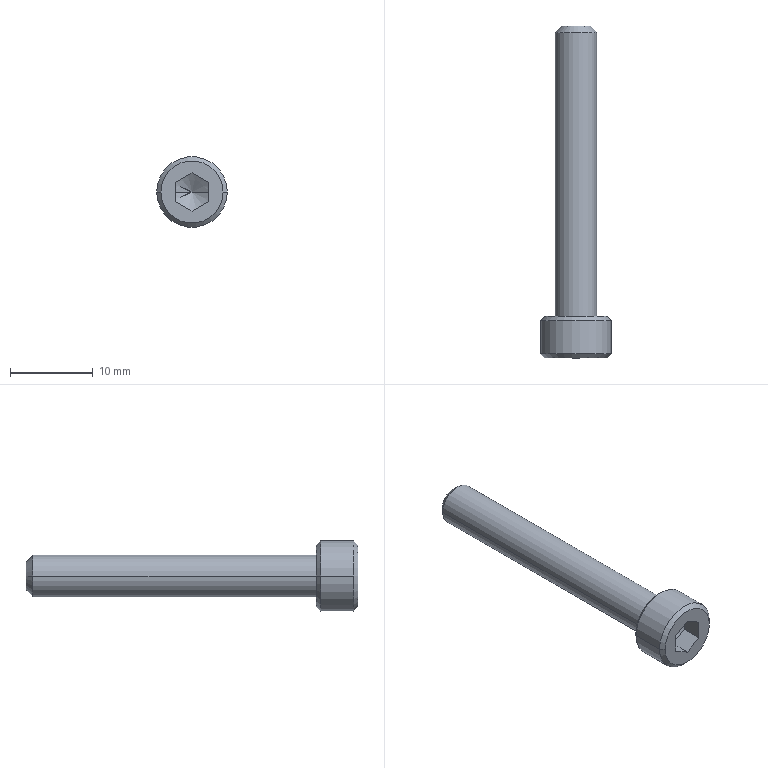Part | STEP file | BB62-M5-35L-3 | 1 solid | 27 faces | box 8.5 x 40 x 8.5 mm | volume 918.722 mm3 | plane 15 | cone 8 | cylinder 4 | commonest cylinder face diameters 5 x2 8.5 x2
STEP:
#1=CARTESIAN_POINT('',(0.,-1.178,0.));
#2=VERTEX_POINT('',#1);
#3=CARTESIAN_POINT('',(2.29,-2.5,0.));
#4=VERTEX_POINT('',#3);
#5=CARTESIAN_POINT('',(0.,-1.178,0.));
#6=DIRECTION('',(0.866,-0.5,0.));
#7=VECTOR('',#6,1000.);
#8=LINE('',#5,#7);
#9=EDGE_CURVE('',#2,#4,#8,.T.);
#10=ORIENTED_EDGE('',*,*,#9,.F.);
#11=CARTESIAN_POINT('',(-2.29,-2.5,0.));
#12=VERTEX_POINT('',#11);
#13=CARTESIAN_POINT('',(0.,-1.178,0.));
#14=DIRECTION('',(-0.866,-0.5,0.));
#15=VECTOR('',#14,1000.);
#16=LINE('',#13,#15);
#17=EDGE_CURVE('',#2,#12,#16,.T.);
#18=ORIENTED_EDGE('',*,*,#17,.T.);
#19=CARTESIAN_POINT('',(-1.983,-2.5,-1.145));
#20=VERTEX_POINT('',#19);
#21=CARTESIAN_POINT('',(0.,-2.5,0.));
#22=DIRECTION('',(0.,-1.,0.));
#23=DIRECTION('',(-1.,0.,0.));
#24=AXIS2_PLACEMENT_3D('',#21,#22,#23);
#25=CIRCLE('',#24,2.29);
#26=EDGE_CURVE('',#12,#20,#25,.T.);
#27=ORIENTED_EDGE('',*,*,#26,.T.);
#28=CARTESIAN_POINT('',(0.,-2.5,-2.29));
#29=VERTEX_POINT('',#28);
#30=CARTESIAN_POINT('',(0.,-2.5,0.));
#31=DIRECTION('',(0.,-1.,0.));
#32=DIRECTION('',(-1.,0.,0.));
#33=AXIS2_PLACEMENT_3D('',#30,#31,#32);
#34=CIRCLE('',#33,2.29);
#35=EDGE_CURVE('',#20,#29,#34,.T.);
#36=ORIENTED_EDGE('',*,*,#35,.T.);
#37=CARTESIAN_POINT('',(1.983,-2.5,-1.145));
#38=VERTEX_POINT('',#37);
#39=CARTESIAN_POINT('',(0.,-2.5,0.));
#40=DIRECTION('',(0.,-1.,0.));
#41=DIRECTION('',(-1.,0.,0.));
#42=AXIS2_PLACEMENT_3D('',#39,#40,#41);
#43=CIRCLE('',#42,2.29);
#44=EDGE_CURVE('',#29,#38,#43,.T.);
#45=ORIENTED_EDGE('',*,*,#44,.T.);
#46=CARTESIAN_POINT('',(0.,-2.5,0.));
#47=DIRECTION('',(0.,-1.,0.));
#48=DIRECTION('',(-1.,0.,0.));
#49=AXIS2_PLACEMENT_3D('',#46,#47,#48);
#50=CIRCLE('',#49,2.29);
#51=EDGE_CURVE('',#38,#4,#50,.T.);
#52=ORIENTED_EDGE('',*,*,#51,.T.);
#53=EDGE_LOOP('',(#10,#18,#27,#36,#45,#52));
#54=FACE_OUTER_BOUND('',#53,.T.);
#55=CARTESIAN_POINT('',(0.,-1001.178,0.));
#56=DIRECTION('',(0.,-1.,0.));
#57=DIRECTION('',(1.,0.,0.));
#58=AXIS2_PLACEMENT_3D('',#55,#56,#57);
#59=CONICAL_SURFACE('',#58,1732.051,1.047);
#60=ADVANCED_FACE('',(#54),#59,.F.);
#61=CARTESIAN_POINT('',(-1.7,35.,0.));
#62=VERTEX_POINT('',#61);
#63=CARTESIAN_POINT('',(1.7,35.,0.));
#64=VERTEX_POINT('',#63);
#65=CARTESIAN_POINT('',(0.,35.,0.));
#66=DIRECTION('',(0.,1.,0.));
#67=DIRECTION('',(1.,0.,0.));
#68=AXIS2_PLACEMENT_3D('',#65,#66,#67);
#69=CIRCLE('',#68,1.7);
#70=EDGE_CURVE('',#62,#64,#69,.T.);
#71=ORIENTED_EDGE('',*,*,#70,.F.);
#72=CARTESIAN_POINT('',(-2.5,34.2,0.));
#73=VERTEX_POINT('',#72);
#74=CARTESIAN_POINT('',(-1.7,35.,0.));
#75=DIRECTION('',(-0.7071,-0.7071,0.));
#76=VECTOR('',#75,1000.);
#77=LINE('',#74,#76);
#78=EDGE_CURVE('',#62,#73,#77,.T.);
#79=ORIENTED_EDGE('',*,*,#78,.T.);
#80=CARTESIAN_POINT('',(2.5,34.2,0.));
#81=VERTEX_POINT('',#80);
#82=CARTESIAN_POINT('',(0.,34.2,0.));
#83=DIRECTION('',(0.,-1.,0.));
#84=DIRECTION('',(-1.,0.,0.));
#85=AXIS2_PLACEMENT_3D('',#82,#83,#84);
#86=CIRCLE('',#85,2.5);
#87=EDGE_CURVE('',#81,#73,#86,.T.);
#88=ORIENTED_EDGE('',*,*,#87,.F.);
#89=CARTESIAN_POINT('',(1.7,35.,0.));
#90=DIRECTION('',(0.7071,-0.7071,0.));
#91=VECTOR('',#90,1000.);
#92=LINE('',#89,#91);
#93=EDGE_CURVE('',#64,#81,#92,.T.);
#94=ORIENTED_EDGE('',*,*,#93,.F.);
#95=EDGE_LOOP('',(#71,#79,#88,#94));
#96=FACE_OUTER_BOUND('',#95,.T.);
#97=CARTESIAN_POINT('',(0.,35.,0.));
#98=DIRECTION('',(0.,-1.,0.));
#99=DIRECTION('',(1.,0.,0.));
#100=AXIS2_PLACEMENT_3D('',#97,#98,#99);
#101=CONICAL_SURFACE('',#100,1.7,0.7854);
#102=ADVANCED_FACE('',(#96),#101,.T.);
#103=ORIENTED_EDGE('',*,*,#87,.T.);
#104=CARTESIAN_POINT('',(-2.5,0.,0.));
#105=VERTEX_POINT('',#104);
#106=CARTESIAN_POINT('',(-2.5,34.2,0.));
#107=DIRECTION('',(0.,-1.,0.));
#108=VECTOR('',#107,1000.);
#109=LINE('',#106,#108);
#110=EDGE_CURVE('',#73,#105,#109,.T.);
#111=ORIENTED_EDGE('',*,*,#110,.T.);
#112=CARTESIAN_POINT('',(2.5,0.,0.));
#113=VERTEX_POINT('',#112);
#114=CARTESIAN_POINT('',(0.,0.,0.));
#115=DIRECTION('',(0.,-1.,0.));
#116=DIRECTION('',(-1.,0.,0.));
#117=AXIS2_PLACEMENT_3D('',#114,#115,#116);
#118=CIRCLE('',#117,2.5);
#119=EDGE_CURVE('',#113,#105,#118,.T.);
#120=ORIENTED_EDGE('',*,*,#119,.F.);
#121=CARTESIAN_POINT('',(2.5,34.2,0.));
#122=DIRECTION('',(0.,-1.,0.));
#123=VECTOR('',#122,1000.);
#124=LINE('',#121,#123);
#125=EDGE_CURVE('',#81,#113,#124,.T.);
#126=ORIENTED_EDGE('',*,*,#125,.F.);
#127=EDGE_LOOP('',(#103,#111,#120,#126));
#128=FACE_OUTER_BOUND('',#127,.T.);
#129=CARTESIAN_POINT('',(0.,34.2,0.));
#130=DIRECTION('',(0.,-1.,0.));
#131=DIRECTION('',(1.,0.,0.));
#132=AXIS2_PLACEMENT_3D('',#129,#130,#131);
#133=CYLINDRICAL_SURFACE('',#132,2.5);
#134=ADVANCED_FACE('',(#128),#133,.T.);
#135=CARTESIAN_POINT('',(3.75,-5.,0.));
#136=VERTEX_POINT('',#135);
#137=CARTESIAN_POINT('',(-3.75,-5.,0.));
#138=VERTEX_POINT('',#137);
#139=CARTESIAN_POINT('',(0.,-5.,0.));
#140=DIRECTION('',(0.,-1.,0.));
#141=DIRECTION('',(-1.,0.,0.));
#142=AXIS2_PLACEMENT_3D('',#139,#140,#141);
#143=CIRCLE('',#142,3.75);
#144=EDGE_CURVE('',#136,#138,#143,.T.);
#145=ORIENTED_EDGE('',*,*,#144,.F.);
#146=CARTESIAN_POINT('',(4.25,-4.5,0.));
#147=VERTEX_POINT('',#146);
#148=CARTESIAN_POINT('',(4.25,-4.5,0.));
#149=DIRECTION('',(0.7071,0.7071,0.));
#150=VECTOR('',#149,1000.);
#151=LINE('',#148,#150);
#152=EDGE_CURVE('',#136,#147,#151,.T.);
#153=ORIENTED_EDGE('',*,*,#152,.T.);
#154=CARTESIAN_POINT('',(-4.25,-4.5,0.));
#155=VERTEX_POINT('',#154);
#156=CARTESIAN_POINT('',(0.,-4.5,0.));
#157=DIRECTION('',(0.,-1.,0.));
#158=DIRECTION('',(-1.,0.,0.));
#159=AXIS2_PLACEMENT_3D('',#156,#157,#158);
#160=CIRCLE('',#159,4.25);
#161=EDGE_CURVE('',#147,#155,#160,.T.);
#162=ORIENTED_EDGE('',*,*,#161,.T.);
#163=CARTESIAN_POINT('',(-4.25,-4.5,0.));
#164=DIRECTION('',(-0.7071,0.7071,0.));
#165=VECTOR('',#164,1000.);
#166=LINE('',#163,#165);
#167=EDGE_CURVE('',#138,#155,#166,.T.);
#168=ORIENTED_EDGE('',*,*,#167,.F.);
#169=EDGE_LOOP('',(#145,#153,#162,#168));
#170=FACE_OUTER_BOUND('',#169,.T.);
#171=CARTESIAN_POINT('',(0.,-4.5,0.));
#172=DIRECTION('',(0.,1.,0.));
#173=DIRECTION('',(-1.,0.,0.));
#174=AXIS2_PLACEMENT_3D('',#171,#172,#173);
#175=CONICAL_SURFACE('',#174,4.25,0.7854);
#176=ADVANCED_FACE('',(#170),#175,.T.);
#177=ORIENTED_EDGE('',*,*,#161,.F.);
#178=CARTESIAN_POINT('',(4.25,-0.5,0.));
#179=VERTEX_POINT('',#178);
#180=CARTESIAN_POINT('',(4.25,-1.62,0.));
#181=DIRECTION('',(0.,1.,0.));
#182=VECTOR('',#181,1000.);
#183=LINE('',#180,#182);
#184=EDGE_CURVE('',#147,#179,#183,.T.);
#185=ORIENTED_EDGE('',*,*,#184,.T.);
#186=CARTESIAN_POINT('',(-4.25,-0.5,0.));
#187=VERTEX_POINT('',#186);
#188=CARTESIAN_POINT('',(0.,-0.5,0.));
#189=DIRECTION('',(0.,-1.,0.));
#190=DIRECTION('',(-1.,0.,0.));
#191=AXIS2_PLACEMENT_3D('',#188,#189,#190);
#192=CIRCLE('',#191,4.25);
#193=EDGE_CURVE('',#179,#187,#192,.T.);
#194=ORIENTED_EDGE('',*,*,#193,.T.);
#195=CARTESIAN_POINT('',(-4.25,-1.62,0.));
#196=DIRECTION('',(0.,1.,0.));
#197=VECTOR('',#196,1000.);
#198=LINE('',#195,#197);
#199=EDGE_CURVE('',#155,#187,#198,.T.);
#200=ORIENTED_EDGE('',*,*,#199,.F.);
#201=EDGE_LOOP('',(#177,#185,#194,#200));
#202=FACE_OUTER_BOUND('',#201,.T.);
#203=CARTESIAN_POINT('',(0.,-1.62,0.));
#204=DIRECTION('',(0.,1.,0.));
#205=DIRECTION('',(-1.,0.,0.));
#206=AXIS2_PLACEMENT_3D('',#203,#204,#205);
#207=CYLINDRICAL_SURFACE('',#206,4.25);
#208=ADVANCED_FACE('',(#202),#207,.T.);
#209=CARTESIAN_POINT('',(3.75,0.,0.));
#210=VERTEX_POINT('',#209);
#211=CARTESIAN_POINT('',(-3.75,0.,0.));
#212=VERTEX_POINT('',#211);
#213=CARTESIAN_POINT('',(0.,0.,0.));
#214=DIRECTION('',(0.,-1.,0.));
#215=DIRECTION('',(-1.,0.,0.));
#216=AXIS2_PLACEMENT_3D('',#213,#214,#215);
#217=CIRCLE('',#216,3.75);
#218=EDGE_CURVE('',#210,#212,#217,.T.);
#219=ORIENTED_EDGE('',*,*,#218,.T.);
#220=CARTESIAN_POINT('',(-3.75,0.,0.));
#221=DIRECTION('',(-0.7071,-0.7071,0.));
#222=VECTOR('',#221,1000.);
#223=LINE('',#220,#222);
#224=EDGE_CURVE('',#212,#187,#223,.T.);
#225=ORIENTED_EDGE('',*,*,#224,.T.);
#226=ORIENTED_EDGE('',*,*,#193,.F.);
#227=CARTESIAN_POINT('',(3.75,0.,0.));
#228=DIRECTION('',(0.7071,-0.7071,0.));
#229=VECTOR('',#228,1000.);
#230=LINE('',#227,#229);
#231=EDGE_CURVE('',#210,#179,#230,.T.);
#232=ORIENTED_EDGE('',*,*,#231,.F.);
#233=EDGE_LOOP('',(#219,#225,#226,#232));
#234=FACE_OUTER_BOUND('',#233,.T.);
#235=CARTESIAN_POINT('',(0.,0.,0.));
#236=DIRECTION('',(0.,-1.,0.));
#237=DIRECTION('',(1.,0.,0.));
#238=AXIS2_PLACEMENT_3D('',#235,#236,#237);
#239=CONICAL_SURFACE('',#238,3.75,0.7854);
#240=ADVANCED_FACE('',(#234),#239,.T.);
#241=CARTESIAN_POINT('',(0.,-5.,0.));
#242=DIRECTION('',(0.,-1.,0.));
#243=DIRECTION('',(-1.,0.,0.));
#244=AXIS2_PLACEMENT_3D('',#241,#242,#243);
#245=CIRCLE('',#244,3.75);
#246=EDGE_CURVE('',#138,#136,#245,.T.);
#247=ORIENTED_EDGE('',*,*,#246,.T.);
#248=ORIENTED_EDGE('',*,*,#144,.T.);
#249=EDGE_LOOP('',(#247,#248));
#250=FACE_OUTER_BOUND('',#249,.T.);
#251=CARTESIAN_POINT('',(0.,-5.,-2.29));
#252=VERTEX_POINT('',#251);
#253=CARTESIAN_POINT('',(-1.983,-5.,-1.145));
#254=VERTEX_POINT('',#253);
#255=CARTESIAN_POINT('',(0.,-5.,-2.29));
#256=DIRECTION('',(-0.866,0.,0.5));
#257=VECTOR('',#256,1000.);
#258=LINE('',#255,#257);
#259=EDGE_CURVE('',#252,#254,#258,.T.);
#260=ORIENTED_EDGE('',*,*,#259,.T.);
#261=CARTESIAN_POINT('',(-1.983,-5.,1.145));
#262=VERTEX_POINT('',#261);
#263=CARTESIAN_POINT('',(-1.983,-5.,-1.145));
#264=DIRECTION('',(0.,0.,1.));
#265=VECTOR('',#264,1000.);
#266=LINE('',#263,#265);
#267=EDGE_CURVE('',#254,#262,#266,.T.);
#268=ORIENTED_EDGE('',*,*,#267,.T.);
#269=CARTESIAN_POINT('',(0.,-5.,2.29));
#270=VERTEX_POINT('',#269);
#271=CARTESIAN_POINT('',(-1.983,-5.,1.145));
#272=DIRECTION('',(0.866,0.,0.5));
#273=VECTOR('',#272,1000.);
#274=LINE('',#271,#273);
#275=EDGE_CURVE('',#262,#270,#274,.T.);
#276=ORIENTED_EDGE('',*,*,#275,.T.);
#277=CARTESIAN_POINT('',(1.983,-5.,1.145));
#278=VERTEX_POINT('',#277);
#279=CARTESIAN_POINT('',(0.,-5.,2.29));
#280=DIRECTION('',(0.866,0.,-0.5));
#281=VECTOR('',#280,1000.);
#282=LINE('',#279,#281);
#283=EDGE_CURVE('',#270,#278,#282,.T.);
#284=ORIENTED_EDGE('',*,*,#283,.T.);
#285=CARTESIAN_POINT('',(1.983,-5.,-1.145));
#286=VERTEX_POINT('',#285);
#287=CARTESIAN_POINT('',(1.983,-5.,1.145));
#288=DIRECTION('',(0.,0.,-1.));
#289=VECTOR('',#288,1000.);
#290=LINE('',#287,#289);
#291=EDGE_CURVE('',#278,#286,#290,.T.);
#292=ORIENTED_EDGE('',*,*,#291,.T.);
#293=CARTESIAN_POINT('',(1.983,-5.,-1.145));
#294=DIRECTION('',(-0.866,0.,-0.5));
#295=VECTOR('',#294,1000.);
#296=LINE('',#293,#295);
#297=EDGE_CURVE('',#286,#252,#296,.T.);
#298=ORIENTED_EDGE('',*,*,#297,.T.);
#299=EDGE_LOOP('',(#260,#268,#276,#284,#292,#298));
#300=FACE_BOUND('',#299,.T.);
#301=CARTESIAN_POINT('',(3.75,-5.,0.));
#302=DIRECTION('',(0.,-1.,0.));
#303=DIRECTION('',(1.,0.,0.));
#304=AXIS2_PLACEMENT_3D('',#301,#302,#303);
#305=PLANE('',#304);
#306=ADVANCED_FACE('',(#250,#300),#305,.T.);
#307=ORIENTED_EDGE('',*,*,#119,.T.);
#308=CARTESIAN_POINT('',(0.,0.,0.));
#309=DIRECTION('',(0.,-1.,0.));
#310=DIRECTION('',(-1.,0.,0.));
#311=AXIS2_PLACEMENT_3D('',#308,#309,#310);
#312=CIRCLE('',#311,2.5);
#313=EDGE_CURVE('',#105,#113,#312,.T.);
#314=ORIENTED_EDGE('',*,*,#313,.T.);
#315=EDGE_LOOP('',(#307,#314));
#316=FACE_BOUND('',#315,.T.);
#317=ORIENTED_EDGE('',*,*,#218,.F.);
#318=CARTESIAN_POINT('',(0.,0.,0.));
#319=DIRECTION('',(0.,-1.,0.));
#320=DIRECTION('',(-1.,0.,0.));
#321=AXIS2_PLACEMENT_3D('',#318,#319,#320);
#322=CIRCLE('',#321,3.75);
#323=EDGE_CURVE('',#212,#210,#322,.T.);
#324=ORIENTED_EDGE('',*,*,#323,.F.);
#325=EDGE_LOOP('',(#317,#324));
#326=FACE_OUTER_BOUND('',#325,.T.);
#327=CARTESIAN_POINT('',(0.,0.,0.));
#328=DIRECTION('',(0.,1.,0.));
#329=DIRECTION('',(-1.,0.,0.));
#330=AXIS2_PLACEMENT_3D('',#327,#328,#329);
#331=PLANE('',#330);
#332=ADVANCED_FACE('',(#316,#326),#331,.T.);
#333=ORIENTED_EDGE('',*,*,#224,.F.);
#334=ORIENTED_EDGE('',*,*,#323,.T.);
#335=ORIENTED_EDGE('',*,*,#231,.T.);
#336=CARTESIAN_POINT('',(0.,-0.5,0.));
#337=DIRECTION('',(0.,-1.,0.));
#338=DIRECTION('',(-1.,0.,0.));
#339=AXIS2_PLACEMENT_3D('',#336,#337,#338);
#340=CIRCLE('',#339,4.25);
#341=EDGE_CURVE('',#187,#179,#340,.T.);
#342=ORIENTED_EDGE('',*,*,#341,.F.);
#343=EDGE_LOOP('',(#333,#334,#335,#342));
#344=FACE_OUTER_BOUND('',#343,.T.);
#345=CARTESIAN_POINT('',(0.,0.,0.));
#346=DIRECTION('',(0.,-1.,0.));
#347=DIRECTION('',(1.,0.,0.));
#348=AXIS2_PLACEMENT_3D('',#345,#346,#347);
#349=CONICAL_SURFACE('',#348,3.75,0.7854);
#350=ADVANCED_FACE('',(#344),#349,.T.);
#351=ORIENTED_EDGE('',*,*,#184,.F.);
#352=CARTESIAN_POINT('',(0.,-4.5,0.));
#353=DIRECTION('',(0.,-1.,0.));
#354=DIRECTION('',(-1.,0.,0.));
#355=AXIS2_PLACEMENT_3D('',#352,#353,#354);
#356=CIRCLE('',#355,4.25);
#357=EDGE_CURVE('',#155,#147,#356,.T.);
#358=ORIENTED_EDGE('',*,*,#357,.F.);
#359=ORIENTED_EDGE('',*,*,#199,.T.);
#360=ORIENTED_EDGE('',*,*,#341,.T.);
#361=EDGE_LOOP('',(#351,#358,#359,#360));
#362=FACE_OUTER_BOUND('',#361,.T.);
#363=CARTESIAN_POINT('',(0.,-1.62,0.));
#364=DIRECTION('',(0.,1.,0.));
#365=DIRECTION('',(-1.,0.,0.));
#366=AXIS2_PLACEMENT_3D('',#363,#364,#365);
#367=CYLINDRICAL_SURFACE('',#366,4.25);
#368=ADVANCED_FACE('',(#362),#367,.T.);
#369=ORIENTED_EDGE('',*,*,#152,.F.);
#370=ORIENTED_EDGE('',*,*,#246,.F.);
#371=ORIENTED_EDGE('',*,*,#167,.T.);
#372=ORIENTED_EDGE('',*,*,#357,.T.);
#373=EDGE_LOOP('',(#369,#370,#371,#372));
#374=FACE_OUTER_BOUND('',#373,.T.);
#375=CARTESIAN_POINT('',(0.,-4.5,0.));
#376=DIRECTION('',(0.,1.,0.));
#377=DIRECTION('',(-1.,0.,0.));
#378=AXIS2_PLACEMENT_3D('',#375,#376,#377);
#379=CONICAL_SURFACE('',#378,4.25,0.7854);
#380=ADVANCED_FACE('',(#374),#379,.T.);
#381=ORIENTED_EDGE('',*,*,#110,.F.);
#382=CARTESIAN_POINT('',(0.,34.2,0.));
#383=DIRECTION('',(0.,-1.,0.));
#384=DIRECTION('',(-1.,0.,0.));
#385=AXIS2_PLACEMENT_3D('',#382,#383,#384);
#386=CIRCLE('',#385,2.5);
#387=EDGE_CURVE('',#73,#81,#386,.T.);
#388=ORIENTED_EDGE('',*,*,#387,.T.);
#389=ORIENTED_EDGE('',*,*,#125,.T.);
#390=ORIENTED_EDGE('',*,*,#313,.F.);
#391=EDGE_LOOP('',(#381,#388,#389,#390));
#392=FACE_OUTER_BOUND('',#391,.T.);
#393=CARTESIAN_POINT('',(0.,34.2,0.));
#394=DIRECTION('',(0.,-1.,0.));
#395=DIRECTION('',(1.,0.,0.));
#396=AXIS2_PLACEMENT_3D('',#393,#394,#395);
#397=CYLINDRICAL_SURFACE('',#396,2.5);
#398=ADVANCED_FACE('',(#392),#397,.T.);
#399=CARTESIAN_POINT('',(0.,35.,0.));
#400=DIRECTION('',(0.,1.,0.));
#401=DIRECTION('',(1.,0.,0.));
#402=AXIS2_PLACEMENT_3D('',#399,#400,#401);
#403=CIRCLE('',#402,1.7);
#404=EDGE_CURVE('',#64,#62,#403,.T.);
#405=ORIENTED_EDGE('',*,*,#404,.T.);
#406=ORIENTED_EDGE('',*,*,#70,.T.);
#407=EDGE_LOOP('',(#405,#406));
#408=FACE_OUTER_BOUND('',#407,.T.);
#409=CARTESIAN_POINT('',(0.,35.,0.));
#410=DIRECTION('',(0.,1.,0.));
#411=DIRECTION('',(-1.,0.,0.));
#412=AXIS2_PLACEMENT_3D('',#409,#410,#411);
#413=PLANE('',#412);
#414=ADVANCED_FACE('',(#408),#413,.T.);
#415=ORIENTED_EDGE('',*,*,#78,.F.);
#416=ORIENTED_EDGE('',*,*,#404,.F.);
#417=ORIENTED_EDGE('',*,*,#93,.T.);
#418=ORIENTED_EDGE('',*,*,#387,.F.);
#419=EDGE_LOOP('',(#415,#416,#417,#418));
#420=FACE_OUTER_BOUND('',#419,.T.);
#421=CARTESIAN_POINT('',(0.,35.,0.));
#422=DIRECTION('',(0.,-1.,0.));
#423=DIRECTION('',(1.,0.,0.));
#424=AXIS2_PLACEMENT_3D('',#421,#422,#423);
#425=CONICAL_SURFACE('',#424,1.7,0.7854);
#426=ADVANCED_FACE('',(#420),#425,.T.);
#427=CARTESIAN_POINT('',(1.983,-2.5,-1.145));
#428=DIRECTION('',(-0.866,0.,-0.5));
#429=VECTOR('',#428,1000.);
#430=LINE('',#427,#429);
#431=EDGE_CURVE('',#38,#29,#430,.T.);
#432=ORIENTED_EDGE('',*,*,#431,.T.);
#433=CARTESIAN_POINT('',(0.,-5.,-2.29));
#434=DIRECTION('',(0.,1.,0.));
#435=VECTOR('',#434,1000.);
#436=LINE('',#433,#435);
#437=EDGE_CURVE('',#252,#29,#436,.T.);
#438=ORIENTED_EDGE('',*,*,#437,.F.);
#439=ORIENTED_EDGE('',*,*,#297,.F.);
#440=CARTESIAN_POINT('',(1.983,-5.,-1.145));
#441=DIRECTION('',(0.,1.,0.));
#442=VECTOR('',#441,1000.);
#443=LINE('',#440,#442);
#444=EDGE_CURVE('',#286,#38,#443,.T.);
#445=ORIENTED_EDGE('',*,*,#444,.T.);
#446=EDGE_LOOP('',(#432,#438,#439,#445));
#447=FACE_OUTER_BOUND('',#446,.T.);
#448=CARTESIAN_POINT('',(1.983,-5.,-1.145));
#449=DIRECTION('',(-0.5,0.,0.866));
#450=DIRECTION('',(0.866,0.,0.5));
#451=AXIS2_PLACEMENT_3D('',#448,#449,#450);
#452=PLANE('',#451);
#453=ADVANCED_FACE('',(#447),#452,.T.);
#454=CARTESIAN_POINT('',(0.,-2.5,-2.29));
#455=DIRECTION('',(-0.866,0.,0.5));
#456=VECTOR('',#455,1000.);
#457=LINE('',#454,#456);
#458=EDGE_CURVE('',#29,#20,#457,.T.);
#459=ORIENTED_EDGE('',*,*,#458,.T.);
#460=CARTESIAN_POINT('',(-1.983,-5.,-1.145));
#461=DIRECTION('',(0.,1.,0.));
#462=VECTOR('',#461,1000.);
#463=LINE('',#460,#462);
#464=EDGE_CURVE('',#254,#20,#463,.T.);
#465=ORIENTED_EDGE('',*,*,#464,.F.);
#466=ORIENTED_EDGE('',*,*,#259,.F.);
#467=ORIENTED_EDGE('',*,*,#437,.T.);
#468=EDGE_LOOP('',(#459,#465,#466,#467));
#469=FACE_OUTER_BOUND('',#468,.T.);
#470=CARTESIAN_POINT('',(0.,-5.,-2.29));
#471=DIRECTION('',(0.5,0.,0.866));
#472=DIRECTION('',(0.866,0.,-0.5));
#473=AXIS2_PLACEMENT_3D('',#470,#471,#472);
#474=PLANE('',#473);
#475=ADVANCED_FACE('',(#469),#474,.T.);
#476=CARTESIAN_POINT('',(-1.983,-2.5,1.145));
#477=VERTEX_POINT('',#476);
#478=CARTESIAN_POINT('',(-1.983,-2.5,-1.145));
#479=DIRECTION('',(0.,0.,1.));
#480=VECTOR('',#479,1000.);
#481=LINE('',#478,#480);
#482=EDGE_CURVE('',#20,#477,#481,.T.);
#483=ORIENTED_EDGE('',*,*,#482,.T.);
#484=CARTESIAN_POINT('',(-1.983,-5.,1.145));
#485=DIRECTION('',(0.,1.,0.));
#486=VECTOR('',#485,1000.);
#487=LINE('',#484,#486);
#488=EDGE_CURVE('',#262,#477,#487,.T.);
#489=ORIENTED_EDGE('',*,*,#488,.F.);
#490=ORIENTED_EDGE('',*,*,#267,.F.);
#491=ORIENTED_EDGE('',*,*,#464,.T.);
#492=EDGE_LOOP('',(#483,#489,#490,#491));
#493=FACE_OUTER_BOUND('',#492,.T.);
#494=CARTESIAN_POINT('',(-1.983,-5.,-1.145));
#495=DIRECTION('',(1.,0.,0.));
#496=DIRECTION('',(0.,0.,-1.));
#497=AXIS2_PLACEMENT_3D('',#494,#495,#496);
#498=PLANE('',#497);
#499=ADVANCED_FACE('',(#493),#498,.T.);
#500=CARTESIAN_POINT('',(0.,-2.5,2.29));
#501=VERTEX_POINT('',#500);
#502=CARTESIAN_POINT('',(-1.983,-2.5,1.145));
#503=DIRECTION('',(0.866,0.,0.5));
#504=VECTOR('',#503,1000.);
#505=LINE('',#502,#504);
#506=EDGE_CURVE('',#477,#501,#505,.T.);
#507=ORIENTED_EDGE('',*,*,#506,.T.);
#508=CARTESIAN_POINT('',(0.,-5.,2.29));
#509=DIRECTION('',(0.,1.,0.));
#510=VECTOR('',#509,1000.);
#511=LINE('',#508,#510);
#512=EDGE_CURVE('',#270,#501,#511,.T.);
#513=ORIENTED_EDGE('',*,*,#512,.F.);
#514=ORIENTED_EDGE('',*,*,#275,.F.);
#515=ORIENTED_EDGE('',*,*,#488,.T.);
#516=EDGE_LOOP('',(#507,#513,#514,#515));
#517=FACE_OUTER_BOUND('',#516,.T.);
#518=CARTESIAN_POINT('',(-1.983,-5.,1.145));
#519=DIRECTION('',(0.5,0.,-0.866));
#520=DIRECTION('',(-0.866,0.,-0.5));
#521=AXIS2_PLACEMENT_3D('',#518,#519,#520);
#522=PLANE('',#521);
#523=ADVANCED_FACE('',(#517),#522,.T.);
#524=CARTESIAN_POINT('',(1.983,-2.5,1.145));
#525=VERTEX_POINT('',#524);
#526=CARTESIAN_POINT('',(0.,-2.5,2.29));
#527=DIRECTION('',(0.866,0.,-0.5));
#528=VECTOR('',#527,1000.);
#529=LINE('',#526,#528);
#530=EDGE_CURVE('',#501,#525,#529,.T.);
#531=ORIENTED_EDGE('',*,*,#530,.T.);
#532=CARTESIAN_POINT('',(1.983,-5.,1.145));
#533=DIRECTION('',(0.,1.,0.));
#534=VECTOR('',#533,1000.);
#535=LINE('',#532,#534);
#536=EDGE_CURVE('',#278,#525,#535,.T.);
#537=ORIENTED_EDGE('',*,*,#536,.F.);
#538=ORIENTED_EDGE('',*,*,#283,.F.);
#539=ORIENTED_EDGE('',*,*,#512,.T.);
#540=EDGE_LOOP('',(#531,#537,#538,#539));
#541=FACE_OUTER_BOUND('',#540,.T.);
#542=CARTESIAN_POINT('',(0.,-5.,2.29));
#543=DIRECTION('',(-0.5,0.,-0.866));
#544=DIRECTION('',(-0.866,0.,0.5));
#545=AXIS2_PLACEMENT_3D('',#542,#543,#544);
#546=PLANE('',#545);
#547=ADVANCED_FACE('',(#541),#546,.T.);
#548=CARTESIAN_POINT('',(1.983,-2.5,1.145));
#549=DIRECTION('',(0.,0.,-1.));
#550=VECTOR('',#549,1000.);
#551=LINE('',#548,#550);
#552=EDGE_CURVE('',#525,#38,#551,.T.);
#553=ORIENTED_EDGE('',*,*,#552,.T.);
#554=ORIENTED_EDGE('',*,*,#444,.F.);
#555=ORIENTED_EDGE('',*,*,#291,.F.);
#556=ORIENTED_EDGE('',*,*,#536,.T.);
#557=EDGE_LOOP('',(#553,#554,#555,#556));
#558=FACE_OUTER_BOUND('',#557,.T.);
#559=CARTESIAN_POINT('',(1.983,-5.,1.145));
#560=DIRECTION('',(-1.,0.,0.));
#561=DIRECTION('',(0.,0.,1.));
#562=AXIS2_PLACEMENT_3D('',#559,#560,#561);
#563=PLANE('',#562);
#564=ADVANCED_FACE('',(#558),#563,.T.);
#565=ORIENTED_EDGE('',*,*,#431,.F.);
#566=ORIENTED_EDGE('',*,*,#44,.F.);
#567=EDGE_LOOP('',(#565,#566));
#568=FACE_OUTER_BOUND('',#567,.T.);
#569=CARTESIAN_POINT('',(0.,-2.5,0.));
#570=DIRECTION('',(0.,-1.,0.));
#571=DIRECTION('',(1.,0.,0.));
#572=AXIS2_PLACEMENT_3D('',#569,#570,#571);
#573=PLANE('',#572);
#574=ADVANCED_FACE('',(#568),#573,.F.);
#575=ORIENTED_EDGE('',*,*,#552,.F.);
#576=CARTESIAN_POINT('',(0.,-2.5,0.));
#577=DIRECTION('',(0.,-1.,0.));
#578=DIRECTION('',(-1.,0.,0.));
#579=AXIS2_PLACEMENT_3D('',#576,#577,#578);
#580=CIRCLE('',#579,2.29);
#581=EDGE_CURVE('',#4,#525,#580,.T.);
#582=ORIENTED_EDGE('',*,*,#581,.F.);
#583=ORIENTED_EDGE('',*,*,#51,.F.);
#584=EDGE_LOOP('',(#575,#582,#583));
#585=FACE_OUTER_BOUND('',#584,.T.);
#586=CARTESIAN_POINT('',(0.,-2.5,0.));
#587=DIRECTION('',(0.,-1.,0.));
#588=DIRECTION('',(1.,0.,0.));
#589=AXIS2_PLACEMENT_3D('',#586,#587,#588);
#590=PLANE('',#589);
#591=ADVANCED_FACE('',(#585),#590,.F.);
#592=ORIENTED_EDGE('',*,*,#530,.F.);
#593=CARTESIAN_POINT('',(0.,-2.5,0.));
#594=DIRECTION('',(0.,-1.,0.));
#595=DIRECTION('',(-1.,0.,0.));
#596=AXIS2_PLACEMENT_3D('',#593,#594,#595);
#597=CIRCLE('',#596,2.29);
#598=EDGE_CURVE('',#525,#501,#597,.T.);
#599=ORIENTED_EDGE('',*,*,#598,.F.);
#600=EDGE_LOOP('',(#592,#599));
#601=FACE_OUTER_BOUND('',#600,.T.);
#602=CARTESIAN_POINT('',(0.,-2.5,0.));
#603=DIRECTION('',(0.,-1.,0.));
#604=DIRECTION('',(1.,0.,0.));
#605=AXIS2_PLACEMENT_3D('',#602,#603,#604);
#606=PLANE('',#605);
#607=ADVANCED_FACE('',(#601),#606,.F.);
#608=ORIENTED_EDGE('',*,*,#506,.F.);
#609=CARTESIAN_POINT('',(0.,-2.5,0.));
#610=DIRECTION('',(0.,-1.,0.));
#611=DIRECTION('',(-1.,0.,0.));
#612=AXIS2_PLACEMENT_3D('',#609,#610,#611);
#613=CIRCLE('',#612,2.29);
#614=EDGE_CURVE('',#501,#477,#613,.T.);
#615=ORIENTED_EDGE('',*,*,#614,.F.);
#616=EDGE_LOOP('',(#608,#615));
#617=FACE_OUTER_BOUND('',#616,.T.);
#618=CARTESIAN_POINT('',(0.,-2.5,0.));
#619=DIRECTION('',(0.,-1.,0.));
#620=DIRECTION('',(1.,0.,0.));
#621=AXIS2_PLACEMENT_3D('',#618,#619,#620);
#622=PLANE('',#621);
#623=ADVANCED_FACE('',(#617),#622,.F.);
#624=ORIENTED_EDGE('',*,*,#482,.F.);
#625=ORIENTED_EDGE('',*,*,#26,.F.);
#626=CARTESIAN_POINT('',(0.,-2.5,0.));
#627=DIRECTION('',(0.,-1.,0.));
#628=DIRECTION('',(-1.,0.,0.));
#629=AXIS2_PLACEMENT_3D('',#626,#627,#628);
#630=CIRCLE('',#629,2.29);
#631=EDGE_CURVE('',#477,#12,#630,.T.);
#632=ORIENTED_EDGE('',*,*,#631,.F.);
#633=EDGE_LOOP('',(#624,#625,#632));
#634=FACE_OUTER_BOUND('',#633,.T.);
#635=CARTESIAN_POINT('',(0.,-2.5,0.));
#636=DIRECTION('',(0.,-1.,0.));
#637=DIRECTION('',(1.,0.,0.));
#638=AXIS2_PLACEMENT_3D('',#635,#636,#637);
#639=PLANE('',#638);
#640=ADVANCED_FACE('',(#634),#639,.F.);
#641=ORIENTED_EDGE('',*,*,#458,.F.);
#642=ORIENTED_EDGE('',*,*,#35,.F.);
#643=EDGE_LOOP('',(#641,#642));
#644=FACE_OUTER_BOUND('',#643,.T.);
#645=CARTESIAN_POINT('',(0.,-2.5,0.));
#646=DIRECTION('',(0.,-1.,0.));
#647=DIRECTION('',(1.,0.,0.));
#648=AXIS2_PLACEMENT_3D('',#645,#646,#647);
#649=PLANE('',#648);
#650=ADVANCED_FACE('',(#644),#649,.F.);
#651=ORIENTED_EDGE('',*,*,#17,.F.);
#652=ORIENTED_EDGE('',*,*,#9,.T.);
#653=ORIENTED_EDGE('',*,*,#581,.T.);
#654=ORIENTED_EDGE('',*,*,#598,.T.);
#655=ORIENTED_EDGE('',*,*,#614,.T.);
#656=ORIENTED_EDGE('',*,*,#631,.T.);
#657=EDGE_LOOP('',(#651,#652,#653,#654,#655,#656));
#658=FACE_OUTER_BOUND('',#657,.T.);
#659=CARTESIAN_POINT('',(0.,-1001.178,0.));
#660=DIRECTION('',(0.,-1.,0.));
#661=DIRECTION('',(1.,0.,0.));
#662=AXIS2_PLACEMENT_3D('',#659,#660,#661);
#663=CONICAL_SURFACE('',#662,1732.051,1.047);
#664=ADVANCED_FACE('',(#658),#663,.F.);
#665=CLOSED_SHELL('',(#60,#102,#134,#176,#208,#240,#306,#332,#350,#368,#380,#398,#414,#426,#453,#475,#499,#523,#547,#564,#574,#591,#607,#623,#640,#650,#664));
#666=MANIFOLD_SOLID_BREP('',#665);
#667=CARTESIAN_POINT('',(0.,0.,0.));
#668=DIRECTION('',(0.,0.,1.));
#669=DIRECTION('',(1.,0.,0.));
#670=AXIS2_PLACEMENT_3D('',#667,#668,#669);
#671=(LENGTH_UNIT()NAMED_UNIT(*)SI_UNIT(.MILLI.,.METRE.));
#672=UNCERTAINTY_MEASURE_WITH_UNIT(LENGTH_MEASURE(0.00001),#671,'','');
#673=(NAMED_UNIT(*)PLANE_ANGLE_UNIT()SI_UNIT($,.RADIAN.));
#674=(NAMED_UNIT(*)SI_UNIT($,.STERADIAN.)SOLID_ANGLE_UNIT());
#675=(GEOMETRIC_REPRESENTATION_CONTEXT(3)GLOBAL_UNCERTAINTY_ASSIGNED_CONTEXT((#672))GLOBAL_UNIT_ASSIGNED_CONTEXT((#671,#673,#674))REPRESENTATION_CONTEXT('',''));
#676=ADVANCED_BREP_SHAPE_REPRESENTATION('',(#666,#670),#675);